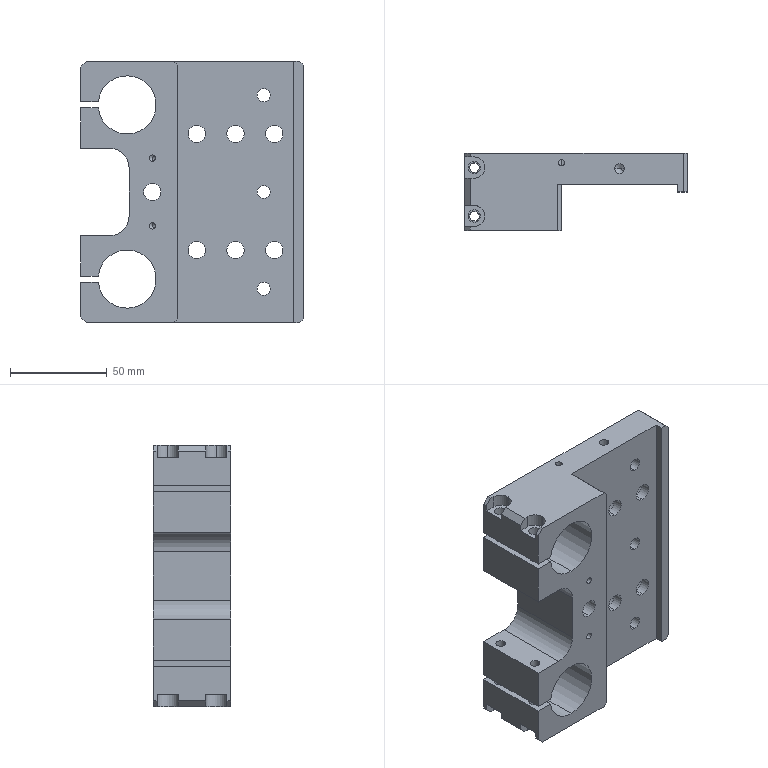Part | SolidWorks | features BaseBody 1 | 1 solid | 155 faces | box 115 x 40 x 135 mm | volume 282474 mm3 | cylinder 88 | plane 51 | cone 16 | commonest cylinder face diameters 5 x16 9 x14 15 x14 3.3 x12 6.4 x8 6.8 x6